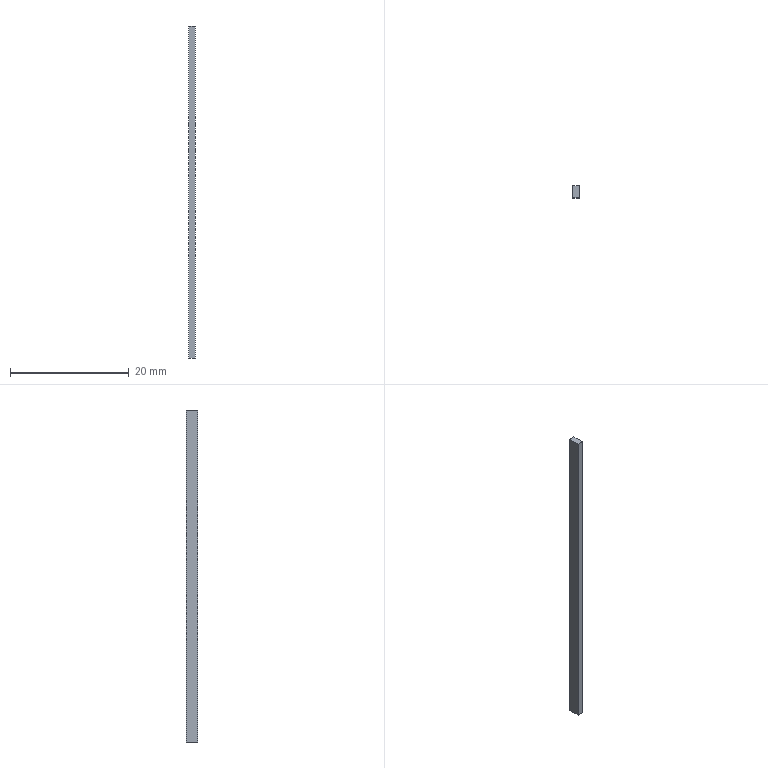Part | NX | features BREP 2 | 2 solids | 12 faces | box 1.02 x 2 x 56 mm | volume 228.503 mm3 | plane 12
STEP:
#1=CARTESIAN_POINT('',(0.5101,1.,-4.));
#2=VERTEX_POINT('',#1);
#3=CARTESIAN_POINT('',(0.5101,1.,52.));
#4=VERTEX_POINT('',#3);
#5=CARTESIAN_POINT('',(0.5101,1.,0.));
#6=DIRECTION('',(0.,0.,1.));
#7=VECTOR('',#6,1000.);
#8=LINE('',#5,#7);
#9=EDGE_CURVE('',#2,#4,#8,.T.);
#10=ORIENTED_EDGE('',*,*,#9,.T.);
#11=CARTESIAN_POINT('',(0.5101,-1.,52.));
#12=VERTEX_POINT('',#11);
#13=CARTESIAN_POINT('',(0.5101,-12.705,52.));
#14=DIRECTION('',(0.,1.,0.));
#15=VECTOR('',#14,1000.);
#16=LINE('',#13,#15);
#17=EDGE_CURVE('',#12,#4,#16,.T.);
#18=ORIENTED_EDGE('',*,*,#17,.F.);
#19=CARTESIAN_POINT('',(0.5101,-1.,-4.));
#20=VERTEX_POINT('',#19);
#21=CARTESIAN_POINT('',(0.5101,-1.,0.));
#22=DIRECTION('',(0.,0.,1.));
#23=VECTOR('',#22,1000.);
#24=LINE('',#21,#23);
#25=EDGE_CURVE('',#20,#12,#24,.T.);
#26=ORIENTED_EDGE('',*,*,#25,.F.);
#27=CARTESIAN_POINT('',(0.5101,-12.705,-4.));
#28=DIRECTION('',(0.,1.,0.));
#29=VECTOR('',#28,1000.);
#30=LINE('',#27,#29);
#31=EDGE_CURVE('',#20,#2,#30,.T.);
#32=ORIENTED_EDGE('',*,*,#31,.T.);
#33=EDGE_LOOP('',(#10,#18,#26,#32));
#34=FACE_BOUND('',#33,.T.);
#35=CARTESIAN_POINT('',(0.5101,1.693,0.));
#36=DIRECTION('',(-1.,0.,0.));
#37=DIRECTION('',(0.,1.,0.));
#38=AXIS2_PLACEMENT_3D('',#35,#36,#37);
#39=PLANE('',#38);
#40=ADVANCED_FACE('',(#34),#39,.F.);
#41=ORIENTED_EDGE('',*,*,#25,.T.);
#42=CARTESIAN_POINT('',(-0.5101,-1.,52.));
#43=VERTEX_POINT('',#42);
#44=CARTESIAN_POINT('',(-10.54,-1.,52.));
#45=DIRECTION('',(1.,0.,0.));
#46=VECTOR('',#45,1000.);
#47=LINE('',#44,#46);
#48=EDGE_CURVE('',#43,#12,#47,.T.);
#49=ORIENTED_EDGE('',*,*,#48,.F.);
#50=CARTESIAN_POINT('',(-0.5101,-1.,-4.));
#51=VERTEX_POINT('',#50);
#52=CARTESIAN_POINT('',(-0.5101,-1.,0.));
#53=DIRECTION('',(0.,0.,1.));
#54=VECTOR('',#53,1000.);
#55=LINE('',#52,#54);
#56=EDGE_CURVE('',#51,#43,#55,.T.);
#57=ORIENTED_EDGE('',*,*,#56,.F.);
#58=CARTESIAN_POINT('',(-10.54,-1.,-4.));
#59=DIRECTION('',(1.,0.,0.));
#60=VECTOR('',#59,1000.);
#61=LINE('',#58,#60);
#62=EDGE_CURVE('',#51,#20,#61,.T.);
#63=ORIENTED_EDGE('',*,*,#62,.T.);
#64=EDGE_LOOP('',(#41,#49,#57,#63));
#65=FACE_BOUND('',#64,.T.);
#66=CARTESIAN_POINT('',(-10.54,-1.,0.));
#67=DIRECTION('',(0.,-1.,0.));
#68=DIRECTION('',(-1.,0.,0.));
#69=AXIS2_PLACEMENT_3D('',#66,#67,#68);
#70=PLANE('',#69);
#71=ADVANCED_FACE('',(#65),#70,.T.);
#72=ORIENTED_EDGE('',*,*,#56,.T.);
#73=CARTESIAN_POINT('',(-0.5101,1.,52.));
#74=VERTEX_POINT('',#73);
#75=CARTESIAN_POINT('',(-0.5101,-12.705,52.));
#76=DIRECTION('',(0.,-1.,0.));
#77=VECTOR('',#76,1000.);
#78=LINE('',#75,#77);
#79=EDGE_CURVE('',#74,#43,#78,.T.);
#80=ORIENTED_EDGE('',*,*,#79,.F.);
#81=CARTESIAN_POINT('',(-0.5101,1.,-4.));
#82=VERTEX_POINT('',#81);
#83=CARTESIAN_POINT('',(-0.5101,1.,0.));
#84=DIRECTION('',(0.,0.,1.));
#85=VECTOR('',#84,1000.);
#86=LINE('',#83,#85);
#87=EDGE_CURVE('',#82,#74,#86,.T.);
#88=ORIENTED_EDGE('',*,*,#87,.F.);
#89=CARTESIAN_POINT('',(-0.5101,-12.705,-4.));
#90=DIRECTION('',(0.,-1.,0.));
#91=VECTOR('',#90,1000.);
#92=LINE('',#89,#91);
#93=EDGE_CURVE('',#82,#51,#92,.T.);
#94=ORIENTED_EDGE('',*,*,#93,.T.);
#95=EDGE_LOOP('',(#72,#80,#88,#94));
#96=FACE_BOUND('',#95,.T.);
#97=CARTESIAN_POINT('',(-0.5101,-10.087,0.));
#98=DIRECTION('',(1.,0.,0.));
#99=DIRECTION('',(0.,-1.,0.));
#100=AXIS2_PLACEMENT_3D('',#97,#98,#99);
#101=PLANE('',#100);
#102=ADVANCED_FACE('',(#96),#101,.F.);
#103=CARTESIAN_POINT('',(-10.54,1.,-4.));
#104=DIRECTION('',(-1.,0.,0.));
#105=VECTOR('',#104,1000.);
#106=LINE('',#103,#105);
#107=EDGE_CURVE('',#2,#82,#106,.T.);
#108=ORIENTED_EDGE('',*,*,#107,.T.);
#109=ORIENTED_EDGE('',*,*,#87,.T.);
#110=CARTESIAN_POINT('',(-10.54,1.,52.));
#111=DIRECTION('',(-1.,0.,0.));
#112=VECTOR('',#111,1000.);
#113=LINE('',#110,#112);
#114=EDGE_CURVE('',#4,#74,#113,.T.);
#115=ORIENTED_EDGE('',*,*,#114,.F.);
#116=ORIENTED_EDGE('',*,*,#9,.F.);
#117=EDGE_LOOP('',(#108,#109,#115,#116));
#118=FACE_BOUND('',#117,.T.);
#119=CARTESIAN_POINT('',(-10.54,1.,0.));
#120=DIRECTION('',(0.,-1.,0.));
#121=DIRECTION('',(-1.,0.,0.));
#122=AXIS2_PLACEMENT_3D('',#119,#120,#121);
#123=PLANE('',#122);
#124=ADVANCED_FACE('',(#118),#123,.F.);
#125=ORIENTED_EDGE('',*,*,#79,.T.);
#126=ORIENTED_EDGE('',*,*,#48,.T.);
#127=ORIENTED_EDGE('',*,*,#17,.T.);
#128=ORIENTED_EDGE('',*,*,#114,.T.);
#129=EDGE_LOOP('',(#125,#126,#127,#128));
#130=FACE_BOUND('',#129,.T.);
#131=CARTESIAN_POINT('',(-10.54,-12.705,52.));
#132=DIRECTION('',(0.,0.,1.));
#133=DIRECTION('',(-1.,0.,0.));
#134=AXIS2_PLACEMENT_3D('',#131,#132,#133);
#135=PLANE('',#134);
#136=ADVANCED_FACE('',(#130),#135,.T.);
#137=ORIENTED_EDGE('',*,*,#93,.F.);
#138=ORIENTED_EDGE('',*,*,#107,.F.);
#139=ORIENTED_EDGE('',*,*,#31,.F.);
#140=ORIENTED_EDGE('',*,*,#62,.F.);
#141=EDGE_LOOP('',(#137,#138,#139,#140));
#142=FACE_BOUND('',#141,.T.);
#143=CARTESIAN_POINT('',(-10.54,-12.705,-4.));
#144=DIRECTION('',(0.,0.,1.));
#145=DIRECTION('',(-1.,0.,0.));
#146=AXIS2_PLACEMENT_3D('',#143,#144,#145);
#147=PLANE('',#146);
#148=ADVANCED_FACE('',(#142),#147,.F.);
#149=CLOSED_SHELL('',(#40,#71,#102,#124,#136,#148));
#150=MANIFOLD_SOLID_BREP('',#149);
#151=CARTESIAN_POINT('',(0.5101,1.,-4.));
#152=VERTEX_POINT('',#151);
#153=CARTESIAN_POINT('',(0.5101,1.,52.));
#154=VERTEX_POINT('',#153);
#155=CARTESIAN_POINT('',(0.5101,1.,0.));
#156=DIRECTION('',(0.,0.,1.));
#157=VECTOR('',#156,1000.);
#158=LINE('',#155,#157);
#159=EDGE_CURVE('',#152,#154,#158,.T.);
#160=ORIENTED_EDGE('',*,*,#159,.T.);
#161=CARTESIAN_POINT('',(0.5101,-1.,52.));
#162=VERTEX_POINT('',#161);
#163=CARTESIAN_POINT('',(0.5101,-12.705,52.));
#164=DIRECTION('',(0.,1.,0.));
#165=VECTOR('',#164,1000.);
#166=LINE('',#163,#165);
#167=EDGE_CURVE('',#162,#154,#166,.T.);
#168=ORIENTED_EDGE('',*,*,#167,.F.);
#169=CARTESIAN_POINT('',(0.5101,-1.,-4.));
#170=VERTEX_POINT('',#169);
#171=CARTESIAN_POINT('',(0.5101,-1.,0.));
#172=DIRECTION('',(0.,0.,1.));
#173=VECTOR('',#172,1000.);
#174=LINE('',#171,#173);
#175=EDGE_CURVE('',#170,#162,#174,.T.);
#176=ORIENTED_EDGE('',*,*,#175,.F.);
#177=CARTESIAN_POINT('',(0.5101,-12.705,-4.));
#178=DIRECTION('',(0.,1.,0.));
#179=VECTOR('',#178,1000.);
#180=LINE('',#177,#179);
#181=EDGE_CURVE('',#170,#152,#180,.T.);
#182=ORIENTED_EDGE('',*,*,#181,.T.);
#183=EDGE_LOOP('',(#160,#168,#176,#182));
#184=FACE_BOUND('',#183,.T.);
#185=CARTESIAN_POINT('',(0.5101,1.693,0.));
#186=DIRECTION('',(-1.,0.,0.));
#187=DIRECTION('',(0.,1.,0.));
#188=AXIS2_PLACEMENT_3D('',#185,#186,#187);
#189=PLANE('',#188);
#190=ADVANCED_FACE('',(#184),#189,.F.);
#191=ORIENTED_EDGE('',*,*,#175,.T.);
#192=CARTESIAN_POINT('',(-0.5101,-1.,52.));
#193=VERTEX_POINT('',#192);
#194=CARTESIAN_POINT('',(-10.54,-1.,52.));
#195=DIRECTION('',(1.,0.,0.));
#196=VECTOR('',#195,1000.);
#197=LINE('',#194,#196);
#198=EDGE_CURVE('',#193,#162,#197,.T.);
#199=ORIENTED_EDGE('',*,*,#198,.F.);
#200=CARTESIAN_POINT('',(-0.5101,-1.,-4.));
#201=VERTEX_POINT('',#200);
#202=CARTESIAN_POINT('',(-0.5101,-1.,0.));
#203=DIRECTION('',(0.,0.,1.));
#204=VECTOR('',#203,1000.);
#205=LINE('',#202,#204);
#206=EDGE_CURVE('',#201,#193,#205,.T.);
#207=ORIENTED_EDGE('',*,*,#206,.F.);
#208=CARTESIAN_POINT('',(-10.54,-1.,-4.));
#209=DIRECTION('',(1.,0.,0.));
#210=VECTOR('',#209,1000.);
#211=LINE('',#208,#210);
#212=EDGE_CURVE('',#201,#170,#211,.T.);
#213=ORIENTED_EDGE('',*,*,#212,.T.);
#214=EDGE_LOOP('',(#191,#199,#207,#213));
#215=FACE_BOUND('',#214,.T.);
#216=CARTESIAN_POINT('',(-10.54,-1.,0.));
#217=DIRECTION('',(0.,-1.,0.));
#218=DIRECTION('',(-1.,0.,0.));
#219=AXIS2_PLACEMENT_3D('',#216,#217,#218);
#220=PLANE('',#219);
#221=ADVANCED_FACE('',(#215),#220,.T.);
#222=ORIENTED_EDGE('',*,*,#206,.T.);
#223=CARTESIAN_POINT('',(-0.5101,1.,52.));
#224=VERTEX_POINT('',#223);
#225=CARTESIAN_POINT('',(-0.5101,-12.705,52.));
#226=DIRECTION('',(0.,-1.,0.));
#227=VECTOR('',#226,1000.);
#228=LINE('',#225,#227);
#229=EDGE_CURVE('',#224,#193,#228,.T.);
#230=ORIENTED_EDGE('',*,*,#229,.F.);
#231=CARTESIAN_POINT('',(-0.5101,1.,-4.));
#232=VERTEX_POINT('',#231);
#233=CARTESIAN_POINT('',(-0.5101,1.,0.));
#234=DIRECTION('',(0.,0.,1.));
#235=VECTOR('',#234,1000.);
#236=LINE('',#233,#235);
#237=EDGE_CURVE('',#232,#224,#236,.T.);
#238=ORIENTED_EDGE('',*,*,#237,.F.);
#239=CARTESIAN_POINT('',(-0.5101,-12.705,-4.));
#240=DIRECTION('',(0.,-1.,0.));
#241=VECTOR('',#240,1000.);
#242=LINE('',#239,#241);
#243=EDGE_CURVE('',#232,#201,#242,.T.);
#244=ORIENTED_EDGE('',*,*,#243,.T.);
#245=EDGE_LOOP('',(#222,#230,#238,#244));
#246=FACE_BOUND('',#245,.T.);
#247=CARTESIAN_POINT('',(-0.5101,-10.087,0.));
#248=DIRECTION('',(1.,0.,0.));
#249=DIRECTION('',(0.,-1.,0.));
#250=AXIS2_PLACEMENT_3D('',#247,#248,#249);
#251=PLANE('',#250);
#252=ADVANCED_FACE('',(#246),#251,.F.);
#253=CARTESIAN_POINT('',(-10.54,1.,-4.));
#254=DIRECTION('',(-1.,0.,0.));
#255=VECTOR('',#254,1000.);
#256=LINE('',#253,#255);
#257=EDGE_CURVE('',#152,#232,#256,.T.);
#258=ORIENTED_EDGE('',*,*,#257,.T.);
#259=ORIENTED_EDGE('',*,*,#237,.T.);
#260=CARTESIAN_POINT('',(-10.54,1.,52.));
#261=DIRECTION('',(-1.,0.,0.));
#262=VECTOR('',#261,1000.);
#263=LINE('',#260,#262);
#264=EDGE_CURVE('',#154,#224,#263,.T.);
#265=ORIENTED_EDGE('',*,*,#264,.F.);
#266=ORIENTED_EDGE('',*,*,#159,.F.);
#267=EDGE_LOOP('',(#258,#259,#265,#266));
#268=FACE_BOUND('',#267,.T.);
#269=CARTESIAN_POINT('',(-10.54,1.,0.));
#270=DIRECTION('',(0.,-1.,0.));
#271=DIRECTION('',(-1.,0.,0.));
#272=AXIS2_PLACEMENT_3D('',#269,#270,#271);
#273=PLANE('',#272);
#274=ADVANCED_FACE('',(#268),#273,.F.);
#275=ORIENTED_EDGE('',*,*,#229,.T.);
#276=ORIENTED_EDGE('',*,*,#198,.T.);
#277=ORIENTED_EDGE('',*,*,#167,.T.);
#278=ORIENTED_EDGE('',*,*,#264,.T.);
#279=EDGE_LOOP('',(#275,#276,#277,#278));
#280=FACE_BOUND('',#279,.T.);
#281=CARTESIAN_POINT('',(-10.54,-12.705,52.));
#282=DIRECTION('',(0.,0.,1.));
#283=DIRECTION('',(-1.,0.,0.));
#284=AXIS2_PLACEMENT_3D('',#281,#282,#283);
#285=PLANE('',#284);
#286=ADVANCED_FACE('',(#280),#285,.T.);
#287=ORIENTED_EDGE('',*,*,#243,.F.);
#288=ORIENTED_EDGE('',*,*,#257,.F.);
#289=ORIENTED_EDGE('',*,*,#181,.F.);
#290=ORIENTED_EDGE('',*,*,#212,.F.);
#291=EDGE_LOOP('',(#287,#288,#289,#290));
#292=FACE_BOUND('',#291,.T.);
#293=CARTESIAN_POINT('',(-10.54,-12.705,-4.));
#294=DIRECTION('',(0.,0.,1.));
#295=DIRECTION('',(-1.,0.,0.));
#296=AXIS2_PLACEMENT_3D('',#293,#294,#295);
#297=PLANE('',#296);
#298=ADVANCED_FACE('',(#292),#297,.F.);
#299=CLOSED_SHELL('',(#190,#221,#252,#274,#286,#298));
#300=MANIFOLD_SOLID_BREP('',#299);
#301=(LENGTH_UNIT()NAMED_UNIT(*)SI_UNIT(.MILLI.,.METRE.));
#302=UNCERTAINTY_MEASURE_WITH_UNIT(LENGTH_MEASURE(0.00001),#301,'','');
#303=(NAMED_UNIT(*)PLANE_ANGLE_UNIT()SI_UNIT($,.RADIAN.));
#304=(NAMED_UNIT(*)SI_UNIT($,.STERADIAN.)SOLID_ANGLE_UNIT());
#305=(GEOMETRIC_REPRESENTATION_CONTEXT(3)GLOBAL_UNCERTAINTY_ASSIGNED_CONTEXT((#302))GLOBAL_UNIT_ASSIGNED_CONTEXT((#301,#303,#304))REPRESENTATION_CONTEXT('',''));
#306=ADVANCED_BREP_SHAPE_REPRESENTATION('',(#150,#300),#305);